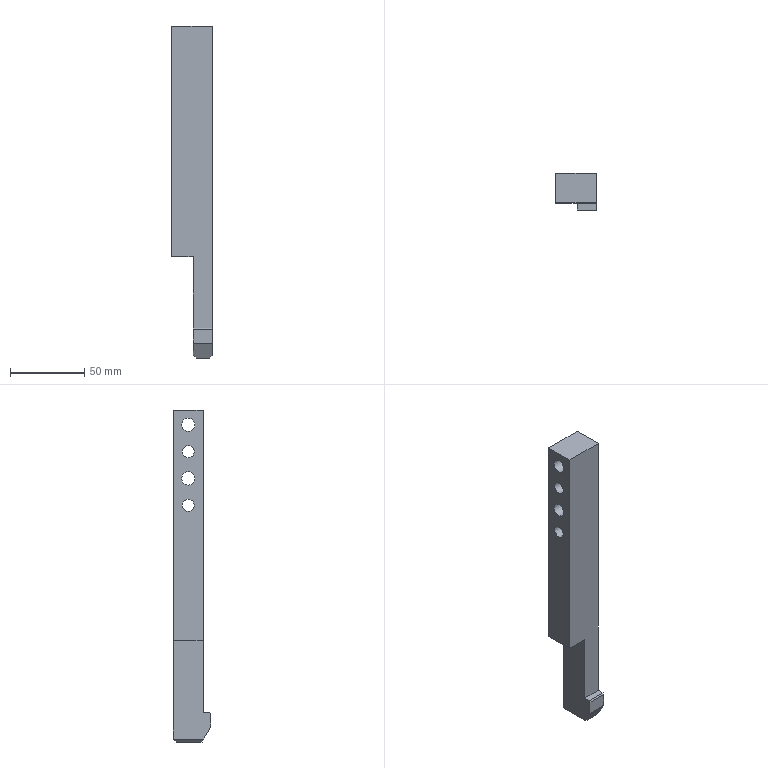Part | STEP file | solid 97 | 1 solid | 23 faces | box 27.5 x 25 x 223 mm | volume 95863 mm3 | plane 17 | cylinder 6 | commonest cylinder face diameters 8 x2 9 x2 14 x2